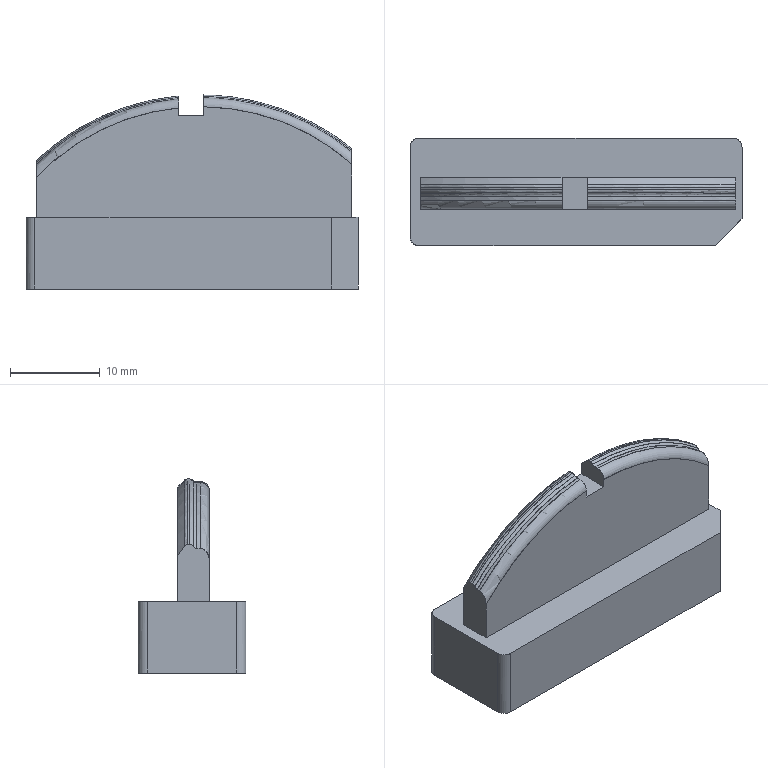NC program | PowerMill | posted with a generic post | part box 37 x 12 x 21.629 mm
Lines 8295 to 9636 of 105205:
N8392 M6
N8393 S18000 M03
N8394 G00 G90 X0.0 Y0.0
N8395 G43 Z9.7988 H28
N8396
N8397 G05 P10000 R4
N8398 X-1.1254 Y1.6882
N8399 Z0.8894
N8400 G01 Z-0.3106 F2400.0
N8401 X-1.1323 Y1.6732 F4000.0
N8402 G03 X-1.06 Y1.4761 I0.1347 J-0.0624
N8403 G01 X-1.0314 Y1.4628
N8404 X-0.7442 Y1.2033
N8405 X-0.6876 Y1.122
N8406 X-0.5772 Y0.8595
N8407 X-0.5402 Y0.5157
N8408 X-0.5342 Y0.1719
N8409 X-0.5752 Y-0.1719
N8410 X-0.6876 Y-0.4228
N8411 X-0.7546 Y-0.5157
N8412 X-1.0314 Y-0.7531
N8413 X-1.0562 Y-0.763
N8414 X0.6776 Y-1.121
N8415 X0.6881 Y-1.1082
N8416 G03 X0.6677 Y-0.8992 I-0.1147 J0.0942
N8417 G01 X0.6193 Y-0.8595
N8418 X0.3669 Y-0.5157
N8419 X0.2839 Y-0.1719
N8420 X0.2975 Y0.8595
N8421 X0.3709 Y1.2033
N8422 X0.6031 Y1.5471
N8423 X0.685 Y1.6182
N8424 G00 Z3.7898
N8425 G01 X0.6171 Y-1.1775 F10000.0
N8426 G00 Z0.7898
N8427 G01 Z-0.4102 F2400.0
N8428 X0.6284 Y-1.1655 F4000.0
N8429 G03 X0.6219 Y-0.9556 I-0.1082 J0.1017
N8430 G01 X0.5196 Y-0.8595
N8431 X0.3438 Y-0.5643
N8432 X0.2794 Y-0.1719
N8433 X0.2975 Y0.8595
N8434 X0.3457 Y1.2033
N8435 X0.5348 Y1.5471
N8436 X0.6741 Y1.6821
N8437 X-0.9646 Y1.7801
N8438 X-0.974 Y1.7665
N8439 G03 X-0.9366 Y1.5599 I0.1221 J-0.0846
N8440 G01 X-0.9181 Y1.5471
N8441 X-0.6445 Y1.2033
N8442 X-0.5496 Y0.8595
N8443 X-0.5471 Y0.5791
N8444 X-0.5402 Y0.5157
N8445 X-0.5342 Y0.1719
N8446 X-0.5428 Y0.1002
N8447 X-0.5404 Y-0.1719
N8448 X-0.6438 Y-0.5157
N8449 X-0.6876 Y-0.5908
N8450 X-0.9294 Y-0.8494
N8451 G00 Z3.6902
N8452 G01 X-0.9561 Y1.9139 F10000.0
N8453 G00 Z0.6902
N8454 G01 Z-0.5098 F2400.0
N8455 X-0.9668 Y1.9014 F4000.0
N8456 G03 X-0.9507 Y1.692 I0.1127 J-0.0966
N8457 G01 X-0.7815 Y1.5471
N8458 X-0.6876 Y1.4155
N8459 X-0.5931 Y1.2033
N8460 X-0.5462 Y0.8595
N8461 X-0.5282 Y-0.1719
N8462 X-0.5744 Y-0.5157
N8463 X-0.6876 Y-0.7569
N8464 X-0.7642 Y-0.8595
N8465 X-0.9273 Y-0.9962
N8466 X0.103 Y-1.2891
N8467 X0.1195 Y-1.2893
N8468 G03 X0.27 Y-1.1428 I0.002 J0.1485
N8469 G01 X0.283 Y-0.1937
N8470 X0.2795 Y-0.1719
N8471 X0.2973 Y0.8443
N8472 X0.2975 Y0.8595
N8473 X0.3438 Y1.3164
N8474 X0.4475 Y1.5471
N8475 X0.6481 Y1.7716
N8476 X-1.0108 Y2.0439 Z-0.6094
N8477 X-1.0221 Y2.0319
N8478 G03 X-1.0159 Y1.822 I0.108 J-0.1019
N8479 G01 X-0.7246 Y1.5471
N8480 X-0.5736 Y1.2033
N8481 X-0.5462 Y0.8595
N8482 X-0.5326 Y0.172
N8483 X-0.5358 Y-0.5157
N8484 X-0.6876 Y-0.9202
N8485 X-0.972 Y-1.2033
N8486 X-1.0951 Y-1.2518
N8487 X0.2983 Y-2.0064
N8488 X0.3128 Y-1.9984
N8489 G03 X0.3708 Y-1.7966 I-0.0719 J0.1299
N8490 G01 X0.3438 Y-1.7478
N8491 X0.2804 Y-1.5471
N8492 X0.2614 Y-1.2033
N8493 X0.2807 Y-0.189
N8494 X0.2805 Y-0.1804
N8495 X0.2795 Y-0.1719
N8496 X0.2973 Y0.8443
N8497 X0.2975 Y0.8595
N8498 X0.3014 Y0.8974
N8499 X0.3072 Y1.2033
N8500 X0.3438 Y1.3884
N8501 X0.4069 Y1.5471
N8502 X0.6876 Y1.8915
N8503 X0.6914 Y1.8935
N8504 X-0.9804 Y2.1178 Z-0.709
N8505 X-0.9922 Y2.1062
N8506 G03 X-0.9937 Y1.8962 I0.1043 J-0.1058
N8507 G01 X-0.6876 Y1.5854
N8508 X-0.5581 Y1.2033
N8509 X-0.5386 Y0.5078
N8510 X-0.5304 Y-0.1879
N8511 X-0.5102 Y-1.2033
N8512 X-0.5414 Y-1.5471
N8513 X-0.5787 Y-1.6288
N8514 X0.3467 Y-2.2202
N8515 X0.3602 Y-2.2108
N8516 G03 X0.397 Y-2.004 I-0.085 J0.1218
N8517 G01 X0.3438 Y-1.9277
N8518 X0.2574 Y-1.5471
N8519 X0.2627 Y-1.2266
N8520 X0.2614 Y-1.2033
N8521 X0.2755 Y-0.4633
N8522 X0.2802 Y-0.1848
N8523 X0.2801 Y-0.1783
N8524 X0.2796 Y-0.1719
N8525 X0.2974 Y0.8443
N8526 X0.2976 Y0.8595
N8527 X0.2977 Y0.8618
N8528 X0.2978 Y0.8641
N8529 X0.3035 Y1.2033
N8530 X0.3438 Y1.482
N8531 X0.5801 Y1.8909
N8532 X0.6876 Y1.9897
N8533 X0.6881 Y1.99
N8534 G00 Z3.3914
N8535 G01 X0.5849 Y-2.5899 F10000.0
N8536 G00 Z0.3914
N8537 G01 Z-0.8086 F2400.0
N8538 X0.5963 Y-2.578 F4000.0
N8539 G03 X0.5923 Y-2.368 I-0.107 J0.103
N8540 G01 X0.4539 Y-2.2347
N8541 X0.3438 Y-2.0504
N8542 X0.288 Y-1.8909
N8543 X0.2554 Y-1.5471
N8544 X0.3035 Y1.2033
N8545 X0.3368 Y1.5471
N8546 X0.4976 Y1.8909
N8547 X0.6854 Y2.0857
N8548 X-0.9959 Y2.214
N8549 X-1.006 Y2.201
N8550 G03 X-0.9805 Y1.9925 I0.117 J-0.0915
N8551 G01 X-0.8505 Y1.8909
N8552 X-0.6876 Y1.6814
N8553 X-0.623 Y1.5471
N8554 X-0.5522 Y1.2033
N8555 X-0.5468 Y0.8667
N8556 X-0.5463 Y0.8595
N8557 X-0.5462 Y0.8541
N8558 X-0.5283 Y-0.1719
N8559 X-0.53 Y-0.1842
N8560 X-0.5276 Y-0.3302
N8561 X-0.5102 Y-1.2033
N8562 X-0.5131 Y-1.2351
N8563 X-0.5081 Y-1.5471
N8564 X-0.5912 Y-1.8909
N8565 X-0.6876 Y-2.0627
N8566 X-0.8419 Y-2.2347
N8567 X-0.8872 Y-2.2667
N8568 G00 Z3.2919
N8569 G01 X-0.988 Y2.313 F10000.0
N8570 G00 Z0.2919
N8571 G01 Z-0.9081 F2400.0
N8572 X-0.999 Y2.3007 F4000.0
N8573 G03 X-0.9878 Y2.091 I0.1104 J-0.0992
N8574 G01 X-0.765 Y1.8909
N8575 X-0.6876 Y1.7773
N8576 X-0.591 Y1.5471
N8577 X-0.5522 Y1.2033
N8578 X-0.5042 Y-1.5471
N8579 X-0.5436 Y-1.8909
N8580 X-0.6876 Y-2.1909
N8581 X-0.9573 Y-2.4285
N8582 X0.6602 Y-2.7332
N8583 X0.6719 Y-2.7215
N8584 G03 Y-2.5115 I-0.105 J0.105
N8585 G01 X0.3953 Y-2.2347
N8586 X0.2673 Y-1.8909
N8587 X0.2554 Y-1.5471
N8588 X0.3035 Y1.2033
N8589 X0.3438 Y1.6691
N8590 X0.4359 Y1.8909
N8591 X0.6774 Y2.1742
N8592 X-0.9835 Y2.4144 Z-1.0077
N8593 X-0.9952 Y2.4028
N8594 G03 X-0.9965 Y2.1928 I0.1043 J-0.1057
N8595 G01 X-0.6984 Y1.8909
N8596 X-0.5705 Y1.5471
N8597 X-0.5522 Y1.2033
N8598 X-0.5042 Y-1.5471
N8599 X-0.5207 Y-1.8909
N8600 X-0.6558 Y-2.2347
N8601 X-0.974 Y-2.5354
N8602 X0.649 Y-2.8215
N8603 X0.6614 Y-2.8107
N8604 G03 X0.6758 Y-2.6011 I-0.0975 J0.112
N8605 G01 X0.3564 Y-2.2347
N8606 X0.2575 Y-1.8909
N8607 X0.2551 Y-1.5921
N8608 X0.2599 Y-1.2934
N8609 X0.3035 Y1.2033
N8610 X0.3042 Y1.2113
N8611 X0.3102 Y1.5471
N8612 X0.3438 Y1.7627
N8613 X0.3886 Y1.8909
N8614 X0.6309 Y2.2347
N8615 X0.6709 Y2.2697
N8616 X-1.001 Y2.5084 Z-1.1073
N8617 X-1.0108 Y2.4951
N8618 G03 X-0.9789 Y2.2875 I0.1197 J-0.0879
N8619 G01 X-0.9071 Y2.2347
N8620 X-0.6876 Y1.9692
N8621 X-0.648 Y1.8909
N8622 X-0.5602 Y1.5471
N8623 X-0.5548 Y1.2513
N8624 X-0.5523 Y1.2033
N8625 X-0.5058 Y-1.4579
N8626 X-0.5042 Y-1.5471
N8627 X-0.5099 Y-1.8909
N8628 X-0.6127 Y-2.2347
N8629 X-0.6876 Y-2.3557
N8630 X-0.906 Y-2.5785
N8631 X-0.9697 Y-2.6191
N8632 X0.7852 Y-2.8878
N8633 X0.7917 Y-2.8727
N8634 G03 X0.7148 Y-2.6772 I-0.1361 J0.0593
N8635 G01 X0.6876 Y-2.6654
N8636 X0.5781 Y-2.5785
N8637 X0.3438 Y-2.2606
N8638 X0.2527 Y-1.8909
N8639 X0.2562 Y-1.6762
N8640 X0.2554 Y-1.5471
N8641 X0.2599 Y-1.2934
N8642 X0.3036 Y1.2033
N8643 X0.3038 Y1.2065
N8644 X0.3039 Y1.2097
N8645 X0.3095 Y1.5471
N8646 X0.3438 Y1.8507
N8647 X0.5422 Y2.2347
N8648 X0.6876 Y2.3767
N8649 X0.6971 Y2.3816
N8650 X-0.9916 Y2.6068 Z-1.2069
N8651 X-1.0023 Y2.5942
N8652 G03 X-0.9856 Y2.3849 I0.113 J-0.0963
N8653 G01 X-0.8093 Y2.2347
N8654 X-0.6876 Y2.0652
N8655 X-0.6104 Y1.8909
N8656 X-0.5582 Y1.5471
N8657 X-0.5101 Y-1.2033
N8658 X-0.5098 Y-1.2322
N8659 X-0.5059 Y-1.4579
N8660 X-0.5042 Y-1.5471
N8661 X-0.5053 Y-1.6107
N8662 X-0.502 Y-1.8909
N8663 X-0.586 Y-2.2347
N8664 X-0.6876 Y-2.4128
N8665 X-0.8369 Y-2.5785
N8666 X-0.9893 Y-2.6843
N8667 X0.7987 Y-2.9338
N8668 X0.8052 Y-2.9186
N8669 G03 X0.7279 Y-2.7234 I-0.1362 J0.0589
N8670 G01 X0.6876 Y-2.7059
N8671 X0.5336 Y-2.5785
N8672 X0.3438 Y-2.3021
N8673 X0.2503 Y-1.8909
N8674 X0.2557 Y-1.5774
N8675 X0.2555 Y-1.5471
N8676 X0.26 Y-1.2934
N8677 X0.2981 Y0.8867
N8678 X0.3095 Y1.5471
N8679 X0.3438 Y1.8507
N8680 X0.5422 Y2.2347
N8681 X0.6876 Y2.3767
N8682 X0.7936 Y2.4316
N8683 G00 Z2.8935
N8684 G01 X0.8024 Y-2.9612 F10000.0
N8685 G00 Z-0.1065
N8686 G01 Z-1.3065 F2400.0
N8687 X0.809 Y-2.946 F4000.0
N8688 G03 X0.7317 Y-2.7508 I-0.1363 J0.0589
N8689 G01 X0.6876 Y-2.7317
N8690 X0.5099 Y-2.5785
N8691 X0.3438 Y-2.3284
N8692 X0.3069 Y-2.2347
N8693 X0.2494 Y-1.8909
N8694 X0.3094 Y1.5471
N8695 X0.3438 Y1.8507
N8696 X0.5422 Y2.2347
N8697 X0.6876 Y2.3767
N8698 X0.7946 Y2.4321
N8699 X-1.0051 Y2.6396
N8700 X-1.0159 Y2.6271
N8701 G03 X-1.0013 Y2.4176 I0.112 J-0.0974
N8702 G01 X-0.791 Y2.2347
N8703 X-0.6876 Y2.0847
N8704 X-0.6042 Y1.8909
N8705 X-0.5581 Y1.5471
N8706 X-0.5547 Y1.3449
N8707 X-0.5102 Y-1.2033
N8708 X-0.5098 Y-1.2322
N8709 X-0.5059 Y-1.4579
N8710 X-0.5043 Y-1.5471
N8711 X-0.5047 Y-1.5686
N8712 X-0.4991 Y-1.8909
N8713 X-0.5685 Y-2.2347
N8714 X-0.6876 Y-2.4559
N8715 X-0.7918 Y-2.5785
N8716 X-0.9912 Y-2.7251
N8717 X0.7845 Y-2.9688 Z-1.4061
N8718 X0.791 Y-2.9537
N8719 G03 X0.7141 Y-2.7583 I-0.1361 J0.0592
N8720 G01 X0.6876 Y-2.7467
N8721 X0.4962 Y-2.5785
N8722 X0.3438 Y-2.3455
N8723 X0.2997 Y-2.2347
N8724 X0.2494 Y-1.8909
N8725 X0.3094 Y1.5471
N8726 X0.3438 Y1.8507
N8727 X0.5422 Y2.2347
N8728 X0.6876 Y2.3767
N8729 X0.7946 Y2.4321
N8730 X-1.0051 Y2.6396
N8731 X-1.0159 Y2.6271
N8732 G03 X-1.0013 Y2.4176 I0.112 J-0.0974
N8733 G01 X-0.791 Y2.2347
N8734 X-0.6876 Y2.0847
N8735 X-0.6042 Y1.8909
N8736 X-0.5581 Y1.5471
N8737 X-0.4982 Y-1.8909
N8738 X-0.5562 Y-2.2347
N8739 X-0.6876 Y-2.4864
N8740 X-0.7634 Y-2.5785
N8741 X-0.9834 Y-2.7481
N8742 X0.788 Y-2.9795 Z-1.5057
N8743 X0.7945 Y-2.9643
N8744 G03 X0.717 Y-2.7691 I-0.1363 J0.0588
N8745 G01 X0.6876 Y-2.7564
N8746 X0.4887 Y-2.5785
N8747 X0.3438 Y-2.354
N8748 X0.2968 Y-2.2347
N8749 X0.2494 Y-1.8909
N8750 X0.3094 Y1.5471
N8751 X0.3438 Y1.8507
N8752 X0.5422 Y2.2347
N8753 X0.6876 Y2.3767
N8754 X0.7946 Y2.4321
N8755 X-1.0051 Y2.6396
N8756 X-1.0159 Y2.6271
N8757 G03 X-1.0013 Y2.4176 I0.112 J-0.0974
N8758 G01 X-0.791 Y2.2347
N8759 X-0.6876 Y2.0847
N8760 X-0.6042 Y1.8909
N8761 X-0.5581 Y1.5471
N8762 X-0.4981 Y-1.8909
N8763 X-0.5499 Y-2.2347
N8764 X-0.6231 Y-2.3626
N8765 X-0.6876 Y-2.4864
N8766 X-0.721 Y-2.5299
N8767 X-0.7465 Y-2.5785
N8768 X-0.9904 Y-2.7693
N8769 G00 Z2.9136
N8770 G01 X-1.0051 Y2.6396 F10000.0
N8771 G00 Z-0.4053
N8772 G01 Z-1.6053 F2400.0
N8773 X-1.0159 Y2.6271 F4000.0
N8774 G03 X-1.0013 Y2.4176 I0.112 J-0.0974
N8775 G01 X-0.791 Y2.2347
N8776 X-0.6876 Y2.0847
N8777 X-0.6042 Y1.8909
N8778 X-0.5581 Y1.5471
N8779 X-0.4981 Y-1.8909
N8780 X-0.5463 Y-2.2347
N8781 X-0.7392 Y-2.5785
N8782 X-0.9902 Y-2.7786
N8783 X0.7918 Y-2.9819
N8784 X0.7984 Y-2.9667
N8785 G03 X0.7209 Y-2.7715 I-0.1364 J0.0588
N8786 G01 X0.6876 Y-2.7572
N8787 X0.488 Y-2.5785
N8788 X0.3438 Y-2.3548
N8789 X0.2965 Y-2.2347
N8790 X0.2494 Y-1.8909
N8791 X0.3094 Y1.5471
N8792 X0.3438 Y1.8507
N8793 X0.5422 Y2.2347
N8794 X0.6876 Y2.3767
N8795 X0.7946 Y2.4321
N8796 X-1.0051 Y2.6396 Z-1.7049
N8797 X-1.0159 Y2.6271
N8798 G03 X-1.0013 Y2.4176 I0.112 J-0.0974
N8799 G01 X-0.791 Y2.2347
N8800 X-0.6876 Y2.0847
N8801 X-0.6041 Y1.8909
N8802 X-0.5581 Y1.5471
N8803 X-0.4981 Y-1.8909
N8804 X-0.5453 Y-2.2347
N8805 X-0.7367 Y-2.5785
N8806 X-0.9902 Y-2.7804
N8807 X0.7932 Y-2.9825
N8808 X0.7997 Y-2.9673
N8809 G03 X0.7222 Y-2.7721 I-0.1363 J0.0588
N8810 G01 X0.6876 Y-2.7572
N8811 X0.488 Y-2.5785
N8812 X0.3438 Y-2.3548
N8813 X0.2965 Y-2.2347
N8814 X0.2494 Y-1.8909
N8815 X0.3094 Y1.5471
N8816 X0.3438 Y1.8508
N8817 X0.5422 Y2.2347
N8818 X0.6876 Y2.3768
N8819 X0.7946 Y2.4321
N8820 X-1.0051 Y2.6396 Z-1.8045
N8821 X-1.0159 Y2.6271
N8822 G03 X-1.0013 Y2.4176 I0.1121 J-0.0974
N8823 G01 X-0.7909 Y2.2347
N8824 X-0.6876 Y2.0847
N8825 X-0.6041 Y1.8909
N8826 X-0.5581 Y1.5471
N8827 X-0.4981 Y-1.8909
N8828 X-0.5453 Y-2.2347
N8829 X-0.7367 Y-2.5785
N8830 X-0.9896 Y-2.7809
N8831 X0.7932 Y-2.9825
N8832 X0.7997 Y-2.9673
N8833 G03 X0.7222 Y-2.7721 I-0.1363 J0.0588
N8834 G01 X0.6876 Y-2.7572
N8835 X0.488 Y-2.5785
N8836 X0.3438 Y-2.3549
N8837 X0.2965 Y-2.2347
N8838 X0.2494 Y-1.8909
N8839 X0.3094 Y1.5471
N8840 X0.3438 Y1.8508
N8841 X0.5422 Y2.2347
N8842 X0.6876 Y2.3768
N8843 X0.7946 Y2.4321
N8844 X-1.0051 Y2.6396 Z-1.9041
N8845 X-1.0159 Y2.6271
N8846 G03 X-1.0013 Y2.4176 I0.1121 J-0.0974
N8847 G01 X-0.7909 Y2.2347
N8848 X-0.6876 Y2.0847
N8849 X-0.6041 Y1.8909
N8850 X-0.5581 Y1.5471
N8851 X-0.4981 Y-1.8909
N8852 X-0.5453 Y-2.2347
N8853 X-0.6876 Y-2.516
N8854 X-0.7176 Y-2.5429
N8855 X-0.7367 Y-2.5785
N8856 X-0.9806 Y-2.7736
N8857 X0.7932 Y-2.9825
N8858 X0.7997 Y-2.9673
N8859 G03 X0.7222 Y-2.7722 I-0.1364 J0.0588
N8860 G01 X0.6876 Y-2.7572
N8861 X0.4879 Y-2.5785
N8862 X0.3438 Y-2.3549
N8863 X0.2965 Y-2.2347
N8864 X0.2494 Y-1.8909
N8865 X0.3094 Y1.5471
N8866 X0.3438 Y1.8508
N8867 X0.5422 Y2.2347
N8868 X0.6876 Y2.3768
N8869 X0.7946 Y2.4321
N8870 G00 Z2.859
N8871 G01 X0.7931 Y-2.9825 F10000.0
N8872 G00 Z-0.8036
N8873 G01 Z-2.0036 F2400.0
N8874 X0.7997 Y-2.9673 F4000.0
N8875 G03 X0.7222 Y-2.7722 I-0.1364 J0.0588
N8876 G01 X0.6876 Y-2.7572
N8877 X0.4879 Y-2.5785
N8878 X0.3438 Y-2.3549
N8879 X0.2965 Y-2.2347
N8880 X0.2494 Y-1.8909
N8881 X0.3094 Y1.5471
N8882 X0.3438 Y1.8508
N8883 X0.5422 Y2.2347
N8884 X0.6876 Y2.3768
N8885 X0.7946 Y2.4321
N8886 X-1.0051 Y2.6396
N8887 X-1.0159 Y2.6271
N8888 G03 X-1.0013 Y2.4176 I0.1121 J-0.0974
N8889 G01 X-0.7909 Y2.2347
N8890 X-0.6876 Y2.0847
N8891 X-0.6041 Y1.8909
N8892 X-0.5581 Y1.5471
N8893 X-0.4981 Y-1.8909
N8894 X-0.5453 Y-2.2347
N8895 X-0.6876 Y-2.5168
N8896 X-0.7176 Y-2.5433
N8897 X-0.7368 Y-2.5784
N8898 X-0.9804 Y-2.7734
N8899 X0.7931 Y-2.9825 Z-2.1033
N8900 X0.7997 Y-2.9674
N8901 G03 X0.7222 Y-2.7722 I-0.1364 J0.0589
N8902 G01 X0.6876 Y-2.7572
N8903 X0.4879 Y-2.5785
N8904 X0.3438 Y-2.3549
N8905 X0.2965 Y-2.2347
N8906 X0.2494 Y-1.8909
N8907 X0.3094 Y1.5471
N8908 X0.3438 Y1.8508
N8909 X0.5422 Y2.2347
N8910 X0.6876 Y2.3768
N8911 X0.7946 Y2.4321
N8912 X-1.0051 Y2.6396
N8913 X-1.0159 Y2.6271
N8914 G03 X-1.0013 Y2.4176 I0.1121 J-0.0974
N8915 G01 X-0.7909 Y2.2347
N8916 X-0.6876 Y2.0848
N8917 X-0.6041 Y1.8909
N8918 X-0.5581 Y1.5471
N8919 X-0.4981 Y-1.8909
N8920 X-0.5453 Y-2.2347
N8921 X-0.6876 Y-2.5176
N8922 X-0.7175 Y-2.5437
N8923 X-0.7368 Y-2.5784
N8924 X-0.9802 Y-2.7732
N8925 G00 Z2.841
N8926 G01 X-1.005 Y2.6396 F10000.0
N8927 G00 Z-1.0028
N8928 G01 Z-2.2028 F2400.0
N8929 X-1.0159 Y2.6271 F4000.0
N8930 G03 X-1.0013 Y2.4176 I0.1121 J-0.0974
N8931 G01 X-0.7909 Y2.2347
N8932 X-0.6876 Y2.0848
N8933 X-0.6041 Y1.8909
N8934 X-0.5581 Y1.5471
N8935 X-0.4981 Y-1.8909
N8936 X-0.5453 Y-2.2347
N8937 X-0.6876 Y-2.5183
N8938 X-0.7175 Y-2.5441
N8939 X-0.7369 Y-2.5784
N8940 X-0.9662 Y-2.7619
N8941 X-0.98 Y-2.774
N8942 X0.7933 Y-2.9826
N8943 X0.7999 Y-2.9674
N8944 G03 X0.7224 Y-2.7723 I-0.1364 J0.0588
N8945 G01 X0.6876 Y-2.7573
N8946 X0.4879 Y-2.5785
N8947 X0.3438 Y-2.3549
N8948 X0.2965 Y-2.2347
N8949 X0.2494 Y-1.8909
N8950 X0.3094 Y1.5471
N8951 X0.3438 Y1.8508
N8952 X0.5422 Y2.2347
N8953 X0.6876 Y2.3768
N8954 X0.7946 Y2.4321
N8955 G00 Z2.9196
N8956 G01 X0.7932 Y-2.9826 F10000.0
N8957 G00 Z-1.1024
N8958 G01 Z-2.3024 F2400.0
N8959 X0.7998 Y-2.9674 F4000.0
N8960 G03 X0.7223 Y-2.7722 I-0.1364 J0.0588
N8961 G01 X0.6876 Y-2.7573
N8962 X0.4879 Y-2.5785
N8963 X0.3438 Y-2.3549
N8964 X0.2965 Y-2.2347
N8965 X0.2494 Y-1.8909
N8966 X0.3094 Y1.5471
N8967 X0.3438 Y1.8508
N8968 X0.5421 Y2.2347
N8969 X0.6876 Y2.3768
N8970 X0.7945 Y2.4321
N8971 X-1.005 Y2.6396
N8972 X-1.0159 Y2.6271
N8973 G03 X-1.0013 Y2.4176 I0.1121 J-0.0974
N8974 G01 X-0.7909 Y2.2347
N8975 X-0.6876 Y2.0848
N8976 X-0.6041 Y1.8909
N8977 X-0.5581 Y1.5471
N8978 X-0.4981 Y-1.8909
N8979 X-0.5453 Y-2.2347
N8980 X-0.6876 Y-2.5191
N8981 X-0.7174 Y-2.5444
N8982 X-0.7369 Y-2.5783
N8983 X-0.9511 Y-2.7498
N8984 X-0.9791 Y-2.7743
N8985 X0.7931 Y-2.9825 Z-2.402
N8986 X0.7997 Y-2.9674
N8987 G03 X0.7222 Y-2.7722 I-0.1364 J0.0589
N8988 G01 X0.6876 Y-2.7573
N8989 X0.4879 Y-2.5785
N8990 X0.3438 Y-2.3549
N8991 X0.2964 Y-2.2347
N8992 X0.2493 Y-1.8909
N8993 X0.3094 Y1.5471
N8994 X0.3438 Y1.8508
N8995 X0.5421 Y2.2347
N8996 X0.6876 Y2.3768
N8997 X0.7945 Y2.4321
N8998 X-1.005 Y2.6396
N8999 X-1.0159 Y2.6271
N9000 G03 X-1.0013 Y2.4176 I0.1121 J-0.0974
N9001 G01 X-0.7909 Y2.2347
N9002 X-0.6876 Y2.0848
N9003 X-0.6041 Y1.8909
N9004 X-0.5581 Y1.5471
N9005 X-0.4981 Y-1.8909
N9006 X-0.5453 Y-2.2347
N9007 X-0.6876 Y-2.5199
N9008 X-0.7173 Y-2.5448
N9009 X-0.7369 Y-2.5783
N9010 X-0.9364 Y-2.7379
N9011 X-0.9782 Y-2.7746
N9012 X0.7945 Y-2.9831 Z-2.5016
N9013 X0.801 Y-2.968
N9014 G03 X0.7235 Y-2.7728 I-0.1363 J0.0589
N9015 G01 X0.6876 Y-2.7573
N9016 X0.4879 Y-2.5785
N9017 X0.3438 Y-2.3549
N9018 X0.2964 Y-2.2347
N9019 X0.2493 Y-1.8909
N9020 X0.3094 Y1.5471
N9021 X0.3438 Y1.8508
N9022 X0.5421 Y2.2347
N9023 X0.6876 Y2.3768
N9024 X0.7945 Y2.4321
N9025 X-1.005 Y2.6396
N9026 X-1.0159 Y2.6271
N9027 G03 X-1.0013 Y2.4176 I0.1121 J-0.0974
N9028 G01 X-0.7909 Y2.2347
N9029 X-0.6876 Y2.0848
N9030 X-0.6041 Y1.8909
N9031 X-0.558 Y1.5471
N9032 X-0.498 Y-1.8909
N9033 X-0.5452 Y-2.2347
N9034 X-0.6876 Y-2.5207
N9035 X-0.7173 Y-2.5452
N9036 X-0.737 Y-2.5783
N9037 X-0.922 Y-2.7264
N9038 X-0.9773 Y-2.7749
N9039 G00 Z9.7988
N9040 G05 P0
N9041 (---------------)
N9042 ( END TOOLPATH : 精公再粗03-外形偏置-D2C )
N9043 (---------------)
N9044
N9045 M05
N9046 G53 Z0.0
N9047 (---------------)
N9048 ( START TOOLPATH : 精公基准台01-基准面偏置-D10 )
N9049 (---------------)
N9050 ( TOOL NO.    :3 )
N9051 ( TOOL TYPE   : ENDMILL)
N9052 ( TOOL ID     : D10_1_1_1)
N9053 ( TOOL DIA    : 10.0 LENGTH 76.8)
N9054 T3
N9055 M6
N9056 S8500 M03
N9057 G00 G90 X0.0 Y0.0
N9058 G43 Z9.7988 H3
N9059
N9060 G05 P10000 R8
N9061 X-8.0986 Y-16.7549
N9062 Z-12.63
N9063 G01 Z-13.83 F360.0
N9064 X-8.0985 Y-11.4798 F600.0
N9065 X0.242 Y-7.3096
N9066 X-17.3097
N9067 X-17.5912 Y-7.3022
N9068 X-17.872 Y-7.2801
N9069 X-18.1513 Y-7.2434
N9070 G02 X-18.7021 Y-7.1263 I1.0414 J6.2539
N9071 G01 X-18.9722 Y-7.0463
N9072 X-19.2377 Y-6.9523
N9073 X-19.4979 Y-6.8445
N9074 G02 X-20.2398 Y-6.4416 I2.3626 J5.2361
N9075 G01 X-20.4719 Y-6.2821
N9076 X-20.6954 Y-6.1106
N9077 X-20.9096 Y-5.9277
N9078 G02 X-21.3078 Y-5.5295 I4.2907 J4.6888
N9079 G01 X-21.4907 Y-5.3154
N9080 X-21.6622 Y-5.0919
N9081 X-21.8217 Y-4.8598
N9082 G02 X-22.1033 Y-4.3721 I5.2818 J3.3745
N9083 G01 X-22.2245 Y-4.1178
N9084 X-22.3323 Y-3.8576
N9085 X-22.4263 Y-3.5921
N9086 X-22.5063 Y-3.322
N9087 X-22.5721 Y-3.0482
N9088 G02 X-22.6602 Y-2.492 I6.1202 J1.2544
N9089 G01 X-22.6823 Y-2.2112
N9090 X-22.6897 Y-1.9296
N9091 Y1.5944
N9092 G02 X-22.6234 Y2.436 I5.7462 J-0.0288
N9093 G01 X-22.5721 Y2.713
N9094 X-22.5063 Y2.9869
N9095 X-22.4263 Y3.2569
N9096 G02 X-22.2245 Y3.7826 I5.9949 J-1.9996
N9097 G01 X-22.1033 Y4.0369
N9098 X-21.9689 Y4.2844
N9099 X-21.8217 Y4.5246
N9100 X-21.6622 Y4.7567
N9101 G02 X-21.3078 Y5.1943 I5.1188 J-3.7827
N9102 G01 X-21.1139 Y5.3986
N9103 X-20.9096 Y5.5925
N9104 X-20.6954 Y5.7755
N9105 X-20.4719 Y5.9469
N9106 X-20.2398 Y6.1064
N9107 X-19.9997 Y6.2536
N9108 X-19.7521 Y6.388
N9109 X-19.4979 Y6.5093
N9110 X-19.2377 Y6.6171
N9111 X-18.9722 Y6.7111
N9112 X-18.7021 Y6.7911
N9113 X-18.4282 Y6.8568
N9114 G02 X-17.872 Y6.9449 I1.2652 J-6.1886
N9115 G01 X-17.5912 Y6.967
N9116 X-17.3097 Y6.9744
N9117 X17.7937
N9118 X18.0752 Y6.967
N9119 X18.356 Y6.9449
N9120 X18.6353 Y6.9082
N9121 X18.9122 Y6.8568
N9122 X19.1861 Y6.7911
N9123 G02 X19.7217 Y6.6171 I-1.6868 J-6.1027
N9124 G01 X19.9819 Y6.5093
N9125 X20.2361 Y6.388
N9126 X20.4837 Y6.2536
N9127 G02 X21.1794 Y5.7754 I-2.8969 J-4.9602
N9128 G01 X21.3936 Y5.5925
N9129 X21.5979 Y5.3986
N9130 X21.7918 Y5.1943
N9131 G02 X22.1462 Y4.7567 I-4.7298 J-4.1924
N9132 G01 X22.3057 Y4.5246
N9133 X22.4529 Y4.2844
N9134 X22.5873 Y4.0369
N9135 G02 X22.8163 Y3.5224 I-5.6007 J-2.8017
N9136 G01 X22.9103 Y3.2569
N9137 X22.9903 Y2.9869
N9138 X23.0561 Y2.713
N9139 X23.1074 Y2.436
N9140 X23.1442 Y2.1568
N9141 G02 X23.1737 Y1.5944 I-6.2063 J-0.6074
N9142 G01 Y-1.9296
N9143 X23.1663 Y-2.2112
N9144 X23.1442 Y-2.492
N9145 G02 X23.0561 Y-3.0482 I-6.412 J0.7305
N9146 G01 X22.9903 Y-3.3221
N9147 X22.9103 Y-3.5921
N9148 X22.8163 Y-3.8576
N9149 X22.7085 Y-4.1178
N9150 G02 X22.4529 Y-4.6196 I-5.7961 J2.6373
N9151 G01 X22.3057 Y-4.8598
N9152 X22.1462 Y-5.0919
N9153 X21.9747 Y-5.3153
N9154 X21.7918 Y-5.5295
N9155 G02 X21.3936 Y-5.9277 I-4.7318 J4.3334
N9156 G01 X21.1794 Y-6.1106
N9157 X20.9559 Y-6.2821
N9158 X20.7238 Y-6.4416
N9159 X20.4837 Y-6.5888
N9160 X20.2361 Y-6.7232
N9161 X19.9819 Y-6.8445
N9162 X19.7217 Y-6.9523
N9163 X19.4562 Y-7.0463
N9164 X19.1861 Y-7.1263
N9165 X18.9122 Y-7.192
N9166 X18.6353 Y-7.2434
N9167 X18.356 Y-7.2801
N9168 G02 X17.7937 Y-7.3096 I-0.619 J6.4337
N9169 G01 X0.242
N9170 G00 Z9.7988
N9171 G05 P0
N9172 (---------------)
N9173 ( END TOOLPATH : 精公基准台01-基准面偏置-D10 )
N9174 (---------------)
N9175 ( START TOOLPATH : 精公基准台01-外形侧光-D10 )
N9176 (---------------)
N9177 G00 X0.0 Y0.0 Z10.799
N9178 G05 P10000 R8
N9179 X20.8332 Y-6.5747
N9180 Z-12.6
N9181 G01 Z-13.8 F360.0
N9182 G03 X19.6852 Y-6.5687 I-0.5813 J-1.3828 F600.0
N9183 G02 X17.708 Y-6.9396 I-1.8939 J4.6408
N9184 G01 X0.1826 Y-6.9395
N9185 X-17.3449
N9186 G02 X-22.3197 Y-1.9168 I0.0353 J5.01
N9187 G01 Y-0.1674
N9188 Y1.5526
N9189 G02 X-17.3428 Y6.6043 I5.0105 J0.0412
N9190 G01 X17.7084 Y6.6044
N9191 G02 X22.8037 Y1.5517 I0.0826 J-5.0121
N9192 G01 Y-1.9181
N9193 G02 X19.6852 Y-6.5687 I-5.0124 J-0.0098
N9194 G03 X18.8691 Y-7.3763 I0.5667 J-1.3888
N9195 G01 X20.7109 Y-6.56
N9196 G03 X19.5632 Y-6.531 I-0.6088 J-1.3709
N9197 G02 X17.708 Y-6.8596 I-1.7719 J4.6031
N9198 G01 X0.1826 Y-6.8595
N9199 X-17.3428
N9200 G02 X-22.2397 Y-1.9168 I0.0332 J4.93
N9201 G01 Y-0.1674
N9202 Y1.5517
N9203 G02 X-17.3428 Y6.5243 I4.9304 J0.0421
N9204 G01 X17.708 Y6.5244
N9205 G02 X22.7237 Y1.5517 I0.083 J-4.9321
N9206 G01 Y-1.9168
N9207 G02 X19.5632 Y-6.531 I-4.9324 J-0.0111
N9208 G03 X18.7312 Y-7.3221 I0.5389 J-1.3999
N9209 G00 Z10.799
N9210 G05 P0
N9211 (---------------)
N9212 ( END TOOLPATH : 精公基准台01-外形侧光-D10 )
N9213 (---------------)
N9214 ( START TOOLPATH : 精公基准台01-基准台侧光-D10 )
N9215 (---------------)
N9216 G00 X0.0 Y0.0 Z9.7988
N9217 G05 P10000 R8
N9218 X23.4954 Y-12.2599
N9219 Z-20.53
N9220 G01 Z-21.73 F360.0
N9221 G03 X19.9599 Y-8.7243 I-1.7678 J1.7678 F600.0
N9222 G01 X19.1433 Y-9.5409
N9223 X19.1431 Y-9.5411
N9224 X19.143 Y-9.5412
N9225 X19.025 Y-9.658
N9226 X19.0238 Y-9.6592
N9227 X19.0225 Y-9.6603
N9228 X18.8028 Y-9.8598
N9229 X18.8015 Y-9.8609
N9230 X18.8002 Y-9.862
N9231 X18.7038 Y-9.9423
N9232 X18.7022 Y-9.9436
N9233 X18.7006 Y-9.9449
N9234 X18.3858 Y-10.1807
N9235 X18.3833 Y-10.1825
N9236 X18.3807 Y-10.1842
N9237 X18.0632 Y-10.3859
N9238 X18.0611 Y-10.3872
N9239 X18.059 Y-10.3884
N9240 X17.8518 Y-10.5028
N9241 X17.8505 Y-10.5035
N9242 X17.8492 Y-10.5042
N9243 X17.7403 Y-10.5593
N9244 X17.7386 Y-10.5602
N9245 X17.7369 Y-10.5609
N9246 X17.4208 Y-10.7028
N9247 X17.4182 Y-10.7039
N9248 X17.4156 Y-10.7049
N9249 X17.0921 Y-10.824
N9250 X17.0896 Y-10.8249
N9251 X17.087 Y-10.8257
N9252 X16.7783 Y-10.9165
N9253 X16.7758 Y-10.9172
N9254 X16.7733 Y-10.9178
N9255 X16.4571 Y-10.989
N9256 X16.4546 Y-10.9895
N9257 X16.4521 Y-10.9899
N9258 X16.1359 Y-11.04
N9259 X16.1334 Y-11.0404
N9260 X16.1309 Y-11.0406
N9261 X15.8147 Y-11.0702
N9262 X15.8122 Y-11.0704
N9263 X15.8097 Y-11.0705
N9264 X15.4935 Y-11.08
N9265 X15.4923
N9266 X15.4911
N9267 X-17.388
N9268 X-17.3885
N9269 X-17.389
N9270 X-17.7052 Y-11.076
N9271 X-17.707
N9272 X-17.7089 Y-11.0759
N9273 X-18.025 Y-11.0573
N9274 X-18.0272 Y-11.0571
N9275 X-18.0294 Y-11.0569
N9276 X-18.3455 Y-11.0209
N9277 X-18.3476 Y-11.0206
N9278 X-18.3497 Y-11.0203
N9279 X-18.6658 Y-10.9671
N9280 X-18.668 Y-10.9668
N9281 X-18.6701 Y-10.9663
N9282 X-18.9862 Y-10.8954
N9283 X-18.9881 Y-10.895
N9284 X-18.99 Y-10.8945
N9285 X-19.2386 Y-10.8261
N9286 X-19.2408 Y-10.8254
N9287 X-19.243 Y-10.8247
N9288 X-19.6266 Y-10.6952
N9289 X-19.6288 Y-10.6944
N9290 X-19.631 Y-10.6935
N9291 X-19.9472 Y-10.5657
N9292 X-19.9487 Y-10.5651
N9293 X-19.9503 Y-10.5644
N9294 X-20.0796 Y-10.5056
N9295 X-20.0808 Y-10.5051
N9296 X-20.082 Y-10.5045
N9297 X-20.2688 Y-10.4119
N9298 X-20.2703 Y-10.4112
N9299 X-20.2717 Y-10.4104
N9300 X-20.5879 Y-10.2374
N9301 X-20.5901 Y-10.2361
N9302 X-20.5923 Y-10.2348
N9303 X-20.9084 Y-10.0347
N9304 X-20.9105 Y-10.0333
N9305 X-20.9126 Y-10.0319
N9306 X-21.2288 Y-9.8023
N9307 X-21.2309 Y-9.8007
N9308 X-21.2329 Y-9.7991
N9309 X-21.5374 Y-9.5459
N9310 X-21.5396 Y-9.544
N9311 X-21.5416 Y-9.5421
N9312 X-21.8694 Y-9.2275
N9313 X-21.8715 Y-9.2255
N9314 X-21.8736 Y-9.2233
N9315 X-22.159 Y-8.9055
N9316 X-22.1607 Y-8.9035
N9317 X-22.1624 Y-8.9014
N9318 X-22.4103 Y-8.5853
N9319 X-22.4116 Y-8.5837
N9320 X-22.4128 Y-8.582
N9321 X-22.5118 Y-8.4414
N9322 X-22.5124 Y-8.4405
N9323 X-22.513 Y-8.4396
N9324 X-22.6294 Y-8.264
N9325 X-22.6305 Y-8.2623
N9326 X-22.6315 Y-8.2606
N9327 X-22.8192 Y-7.9445
N9328 X-22.8204 Y-7.9424
N9329 X-22.8215 Y-7.9403
N9330 X-22.9845 Y-7.6242
N9331 X-22.9856 Y-7.622
N9332 X-22.9865 Y-7.6199
N9333 X-23.1266 Y-7.3038
N9334 X-23.1275 Y-7.3017
N9335 X-23.1283 Y-7.2995
N9336 X-23.2474 Y-6.9834
N9337 X-23.2481 Y-6.9813
N9338 X-23.2488 Y-6.9792
N9339 X-23.348 Y-6.663
N9340 X-23.3487 Y-6.6609
N9341 X-23.3492 Y-6.6588
N9342 X-23.4298 Y-6.3427
N9343 X-23.4303 Y-6.3409
N9344 X-23.4307 Y-6.3391
N9345 X-23.4731 Y-6.1333
N9346 X-23.4735 Y-6.1313
N9347 X-23.4739 Y-6.1293
N9348 X-23.5391 Y-5.7027
N9349 X-23.5395 Y-5.7001
N9350 X-23.5398 Y-5.6975
N9351 X-23.567 Y-5.3813
N9352 X-23.5672 Y-5.3795
N9353 X-23.5673 Y-5.3776
N9354 X-23.5796 Y-5.0615
N9355 Y-5.0599
N9356 X-23.5797 Y-5.0583
N9357 Y5.0583
N9358 Y5.0598
N9359 X-23.5796 Y5.0612
N9360 X-23.5683 Y5.3773
N9361 X-23.5682 Y5.3795
N9362 X-23.568 Y5.3816
N9363 X-23.5398 Y5.6977
N9364 X-23.5395 Y5.6998
N9365 X-23.5393 Y5.7019
N9366 X-23.4941 Y6.0181
N9367 X-23.4938 Y6.0202
N9368 X-23.4934 Y6.0223
N9369 X-23.4307 Y6.3385
N9370 X-23.4303 Y6.3406
N9371 X-23.4298 Y6.3427
N9372 X-23.3492 Y6.6588
N9373 X-23.3486 Y6.6609
N9374 X-23.348 Y6.663
N9375 X-23.2487 Y6.9792
N9376 X-23.2481 Y6.9811
N9377 X-23.2474 Y6.983
N9378 X-23.1537 Y7.2362
N9379 X-23.1528 Y7.2383
N9380 X-23.152 Y7.2404
N9381 X-22.9866 Y7.6195
N9382 X-22.9856 Y7.6218
N9383 X-22.9845 Y7.624
N9384 X-22.8337 Y7.9179
N9385 X-22.8326 Y7.92
N9386 X-22.8314 Y7.9221
N9387 X-22.6316 Y8.2605
N9388 X-22.6306 Y8.2622
N9389 X-22.6295 Y8.2639
N9390 X-22.5131 Y8.4402
N9391 X-22.5124 Y8.4413
N9392 X-22.5116 Y8.4423
N9393 X-22.4127 Y8.5821
N9394 X-22.4117 Y8.5836
N9395 X-22.4106 Y8.585
N9396 X-22.1934 Y8.8649
N9397 X-22.1917 Y8.867
N9398 X-22.1899 Y8.8691
N9399 X-21.8754 Y9.2215
N9400 X-21.8733 Y9.2237
N9401 X-21.8712 Y9.2259
N9402 X-21.5534 Y9.5317
N9403 X-21.5513 Y9.5336
N9404 X-21.5491 Y9.5355
N9405 X-21.233 Y9.799
N9406 X-21.2316 Y9.8001
N9407 X-21.2303 Y9.8012
N9408 X-21.1477 Y9.8641
N9409 X-21.1466 Y9.8649
N9410 X-21.1455 Y9.8657
N9411 X-20.9119 Y10.0316
N9412 X-20.9102 Y10.0328
N9413 X-20.9085 Y10.0339
N9414 X-20.5924 Y10.2347
N9415 X-20.5902 Y10.2361
N9416 X-20.588 Y10.2373
N9417 X-20.2719 Y10.4112
N9418 X-20.2702 Y10.4121
N9419 X-20.2686 Y10.4129
N9420 X-20.0817 Y10.5046
N9421 X-20.0807 Y10.5051
N9422 X-20.0796 Y10.5056
N9423 X-19.9503 Y10.5644
N9424 X-19.9488 Y10.565
N9425 X-19.9473 Y10.5657
N9426 X-19.6312 Y10.6942
N9427 X-19.6291 Y10.695
N9428 X-19.6269 Y10.6958
N9429 X-19.3108 Y10.804
N9430 X-19.3087 Y10.8047
N9431 X-19.3066 Y10.8053
N9432 X-18.9904 Y10.8943
N9433 X-18.9883 Y10.8949
N9434 X-18.9862 Y10.8954
N9435 X-18.6701 Y10.9662
N9436 X-18.668 Y10.9666
N9437 X-18.6659 Y10.967
N9438 X-18.3497 Y11.0203
N9439 X-18.3476 Y11.0206
N9440 X-18.3455 Y11.0209
N9441 X-18.0293 Y11.0567
N9442 X-18.0272 Y11.057
N9443 X-18.025 Y11.0571
N9444 X-17.7089 Y11.0757
N9445 X-17.707 Y11.0758
N9446 X-17.7052
N9447 X-17.3891 Y11.08
N9448 X-17.3885
N9449 X-17.388
N9450 X0.0
N9451 X17.388
N9452 X17.3885
N9453 X17.389
N9454 X17.7052 Y11.076
N9455 X17.707
N9456 X17.7089 Y11.0759
N9457 X18.025 Y11.0573
N9458 X18.0272 Y11.0571
N9459 X18.0294 Y11.0569
N9460 X18.3455 Y11.0209
N9461 X18.3476 Y11.0206
N9462 X18.3497 Y11.0203
N9463 X18.6658 Y10.9672
N9464 X18.668 Y10.9668
N9465 X18.6701 Y10.9663
N9466 X18.9862 Y10.8954
N9467 X18.9881 Y10.895
N9468 X18.99 Y10.8945
N9469 X19.2386 Y10.8261
N9470 X19.2408 Y10.8254
N9471 X19.243 Y10.8247
N9472 X19.6266 Y10.6951
N9473 X19.6288 Y10.6944
N9474 X19.631 Y10.6935
N9475 X19.9472 Y10.5657
N9476 X19.9487 Y10.5651
N9477 X19.9503 Y10.5644
N9478 X20.0796 Y10.5056
N9479 X20.0808 Y10.5051
N9480 X20.082 Y10.5045
N9481 X20.2688 Y10.4119
N9482 X20.2703 Y10.4112
N9483 X20.2717 Y10.4104
N9484 X20.5879 Y10.2374
N9485 X20.5901 Y10.2361
N9486 X20.5923 Y10.2348
N9487 X20.9084 Y10.0347
N9488 X20.9105 Y10.0333
N9489 X20.9126 Y10.0319
N9490 X21.2288 Y9.8023
N9491 X21.2309 Y9.8007
N9492 X21.2329 Y9.7991
N9493 X21.5374 Y9.5459
N9494 X21.5396 Y9.544
N9495 X21.5416 Y9.5421
N9496 X21.8694 Y9.2276
N9497 X21.8715 Y9.2255
N9498 X21.8736 Y9.2233
N9499 X22.159 Y8.9055
N9500 X22.1607 Y8.9035
N9501 X22.1624 Y8.9014
N9502 X22.4103 Y8.5853
N9503 X22.4116 Y8.5837
N9504 X22.4128 Y8.582
N9505 X22.5118 Y8.4414
N9506 X22.5124 Y8.4405
N9507 X22.513 Y8.4396
N9508 X22.6294 Y8.264
N9509 X22.6305 Y8.2623
N9510 X22.6315 Y8.2606
N9511 X22.8192 Y7.9445
N9512 X22.8204 Y7.9424
N9513 X22.8215 Y7.9403
N9514 X22.9845 Y7.6242
N9515 X22.9856 Y7.622
N9516 X22.9865 Y7.6199
N9517 X23.1266 Y7.3038
N9518 X23.1275 Y7.3017
N9519 X23.1283 Y7.2995
N9520 X23.2474 Y6.9834
N9521 X23.2481 Y6.9813
N9522 X23.2488 Y6.9792
N9523 X23.348 Y6.663
N9524 X23.3487 Y6.6609
N9525 X23.3492 Y6.6588
N9526 X23.4298 Y6.3427
N9527 X23.4303 Y6.3409
N9528 X23.4307 Y6.3391
N9529 X23.4731 Y6.1333
N9530 X23.4735 Y6.1313
N9531 X23.4739 Y6.1293
N9532 X23.5391 Y5.7027
N9533 X23.5395 Y5.7001
N9534 X23.5398 Y5.6975
N9535 X23.567 Y5.3813
N9536 X23.5672 Y5.3795
N9537 X23.5673 Y5.3776
N9538 X23.5796 Y5.0615
N9539 X23.5797 Y5.0599
N9540 Y5.0583
N9541 X23.58 Y-2.8453
N9542 Y-2.8456
N9543 Y-2.846
N9544 X23.5774 Y-3.1621
N9545 X23.5773 Y-3.1643
N9546 X23.5772 Y-3.1666
N9547 X23.557 Y-3.4827
N9548 X23.5568 Y-3.4853
N9549 X23.5565 Y-3.4878
N9550 X23.516 Y-3.8039
N9551 X23.5156 Y-3.8065
N9552 X23.5151 Y-3.809
N9553 X23.4538 Y-4.1251
N9554 X23.4533 Y-4.1277
N9555 X23.4526 Y-4.1302
N9556 X23.3697 Y-4.4463
N9557 X23.369 Y-4.4489
N9558 X23.3682 Y-4.4514
N9559 X23.2625 Y-4.7675
N9560 X23.2617 Y-4.7699
N9561 X23.2608 Y-4.7722
N9562 X23.1528 Y-5.039
N9563 X23.1517 Y-5.0416
N9564 X23.1505 Y-5.0441
N9565 X22.9721 Y-5.4096
N9566 X22.9709 Y-5.412
N9567 X22.9695 Y-5.4144
N9568 X22.8318 Y-5.6536
N9569 X22.8311 Y-5.6549
N9570 X22.8303 Y-5.6561
N9571 X22.7821 Y-5.7331
N9572 X22.7811 Y-5.7347
N9573 X22.7801 Y-5.7362
N9574 X22.5606 Y-6.0524
N9575 X22.5596 Y-6.0539
N9576 X22.5585 Y-6.0554
N9577 X22.5099 Y-6.1189
N9578 X22.5089 Y-6.1202
N9579 X22.5078 Y-6.1214
N9580 X22.2976 Y-6.3741
N9581 X22.2963 Y-6.3756
N9582 X22.295 Y-6.377
N9583 X22.1891 Y-6.4924
N9584 X22.1881 Y-6.4934
N9585 X22.1871 Y-6.4945
N9586 X21.989 Y-6.6953
N9587 X21.9888 Y-6.6954
N9588 X21.9886 Y-6.6956
N9589 X19.9599 Y-8.7243
N9590 G03 X23.4954 Y-12.2599 I1.7677 J-1.7678
N9591 G01 X23.4441 Y-12.198
N9592 G03 X19.9086 Y-8.6625 I-1.7677 J1.7677
N9593 G01 X19.0867 Y-9.4844
N9594 X18.9687 Y-9.6011
N9595 X18.749 Y-9.8005
N9596 X18.6526 Y-9.8809
N9597 X18.3378 Y-10.1167
N9598 X18.0203 Y-10.3183
N9599 X17.8131 Y-10.4328
N9600 X17.7042 Y-10.488
N9601 X17.388 Y-10.6298
N9602 X17.0644 Y-10.749
N9603 X16.7557 Y-10.8398
N9604 X16.4396 Y-10.9109
N9605 X16.1234 Y-10.961
N9606 X15.8073 Y-10.9906
N9607 X15.4911 Y-11.0
N9608 X-17.388
N9609 X-17.7042 Y-10.996
N9610 X-18.0203 Y-10.9774
N9611 X-18.3364 Y-10.9414
N9612 X-18.6526 Y-10.8882
N9613 X-18.9687 Y-10.8174
N9614 X-19.2174 Y-10.749
N9615 X-19.601 Y-10.6194
N9616 X-19.9172 Y-10.4916
N9617 X-20.0465 Y-10.4328
N9618 X-20.2333 Y-10.3402
N9619 X-20.5495 Y-10.1672
N9620 X-20.8656 Y-9.9671
N9621 X-21.1818 Y-9.7376
N9622 X-21.4862 Y-9.4844
N9623 X-21.8141 Y-9.1698
N9624 X-22.0995 Y-8.8521
N9625 X-22.3474 Y-8.5359
N9626 X-22.4463 Y-8.3954
N9627 X-22.5627 Y-8.2198
N9628 X-22.7504 Y-7.9036
N9629 X-22.9134 Y-7.5875
N9630 X-23.0535 Y-7.2714
N9631 X-23.1725 Y-6.9552
N9632 X-23.2717 Y-6.6391
N9633 X-23.3523 Y-6.3229
N9634 X-23.3948 Y-6.1172
N9635 X-23.4601 Y-5.6906
N9636 X-23.4873 Y-5.3745
N9637 X-23.4997 Y-5.0583
N9638 Y5.0583
N9639 X-23.4883 Y5.3745
N9640 X-23.4601 Y5.6906
N9641 X-23.4149 Y6.0068
N9642 X-23.3523 Y6.3229
N9643 X-23.2717 Y6.6391
N9644 X-23.1724 Y6.9552
N9645 X-23.0786 Y7.2084
N9646 X-22.9133 Y7.5875
N9647 X-22.7625 Y7.8814
N9648 X-22.5627 Y8.2198
N9649 X-22.4463 Y8.3961
N9650 X-22.3474 Y8.5359
N9651 X-22.1302 Y8.8159
N9652 X-21.8157 Y9.1682
N9653 X-21.4979 Y9.474
N9654 X-21.1818 Y9.7376
N9655 X-21.0992 Y9.8005
N9656 X-20.8656 Y9.9664
N9657 X-20.5495 Y10.1672
N9658 X-20.2333 Y10.3411
N9659 X-20.0465 Y10.4328
N9660 X-19.9172 Y10.4916
N9661 X-19.601 Y10.6201
N9662 X-19.2849 Y10.7283
N9663 X-18.9687 Y10.8173
N9664 X-18.6526 Y10.8881
N9665 X-18.3364 Y10.9414
N9666 X-18.0203 Y10.9772
N9667 X-17.7042 Y10.9958
N9668 X-17.388 Y11.0
N9669 X0.0
N9670 X17.388
N9671 X17.7042 Y10.996
N9672 X18.0203 Y10.9774
N9673 X18.3364 Y10.9414
N9674 X18.6526 Y10.8883
N9675 X18.9687 Y10.8174
N9676 X19.2174 Y10.749
N9677 X19.601 Y10.6194
N9678 X19.9172 Y10.4916
N9679 X20.0465 Y10.4328
N9680 X20.2333 Y10.3402
N9681 X20.5495 Y10.1672
N9682 X20.8656 Y9.9671
N9683 X21.1818 Y9.7376
N9684 X21.4862 Y9.4844
N9685 X21.8141 Y9.1698
N9686 X22.0995 Y8.8521
N9687 X22.3474 Y8.5359
N9688 X22.4463 Y8.3954
N9689 X22.5627 Y8.2198
N9690 X22.7504 Y7.9036
N9691 X22.9134 Y7.5875
N9692 X23.0535 Y7.2714
N9693 X23.1725 Y6.9552
N9694 X23.2717 Y6.6391
N9695 X23.3523 Y6.3229
N9696 X23.3948 Y6.1172
N9697 X23.4601 Y5.6906
N9698 X23.4873 Y5.3745
N9699 X23.4997 Y5.0583
N9700 X23.5 Y-2.8453
N9701 X23.4974 Y-3.1615
N9702 X23.4771 Y-3.4776
N9703 X23.4366 Y-3.7937
N9704 X23.3753 Y-4.1099
N9705 X23.2923 Y-4.426
N9706 X23.1867 Y-4.7422
N9707 X23.0786 Y-5.009
N9708 X22.9002 Y-5.3745
N9709 X22.7625 Y-5.6137
N9710 X22.7143 Y-5.6906
N9711 X22.4949 Y-6.0068
N9712 X22.4463 Y-6.0703
N9713 X22.2361 Y-6.3229
N9714 X22.1302 Y-6.4383
N9715 X21.932 Y-6.6391
N9716 X19.9086 Y-8.6625
N9717 G03 X23.4441 Y-12.198 I1.7678 J-1.7678
N9718 G00 Z9.7988
N9719 G05 P0
N9720 (---------------)
N9721 ( END TOOLPATH : 精公基准台01-基准台侧光-D10 )
N9722 (---------------)
N9723
N9724 M05
N9725 G53 Z0.0
N9726 (---------------)
N9727 ( START TOOLPATH : 精公精光01-平行-R1 )
N9728 (---------------)
N9729 ( TOOL NO.    :4 )
N9730 ( TOOL TYPE   : BALLNOSED)
N9731 ( TOOL ID     : R1_1_1)
N9732 ( TOOL DIA    : 2.0 LENGTH 65.24)
N9733 T4